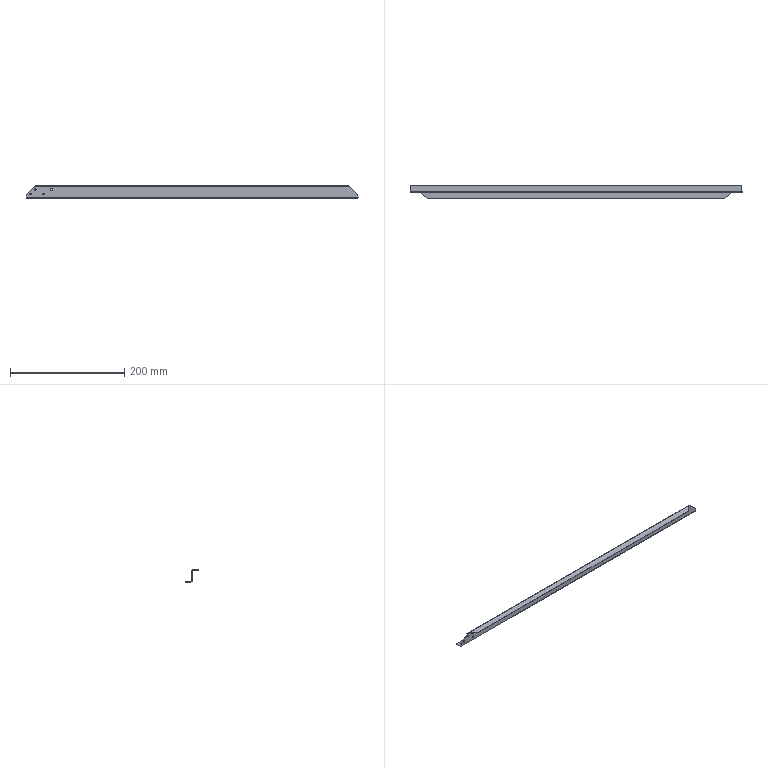Part | SolidWorks | features BaseBody 1 | 1 solid | 28 faces | box 580 x 23.255 x 21.213 mm | volume 12071 mm3 | plane 14 | cylinder 12 | spline 2 | commonest cylinder face diameters 3.2 x8 2 x2 3 x2
STEP:
#1=CARTESIAN_POINT('',(-245.299,-9.6,-7.68));
#2=VERTEX_POINT('',#1);
#3=CARTESIAN_POINT('',(-245.299,-9.556,-4.48));
#4=VERTEX_POINT('',#3);
#5=CARTESIAN_POINT('',(-245.299,-9.578,-6.08));
#6=DIRECTION('',(0.,0.9999,-0.01396));
#7=DIRECTION('',(0.,-0.01396,-0.9999));
#8=AXIS2_PLACEMENT_3D('',#5,#6,#7);
#9=CIRCLE('',#8,1.6);
#10=EDGE_CURVE('',#2,#4,#9,.T.);
#11=ORIENTED_EDGE('',*,*,#10,.T.);
#12=CARTESIAN_POINT('',(-245.299,-10.055,-4.473));
#13=VERTEX_POINT('',#12);
#14=CARTESIAN_POINT('',(-245.299,-9.556,-4.48));
#15=DIRECTION('',(0.,-0.9999,0.01396));
#16=VECTOR('',#15,1000.);
#17=LINE('',#14,#16);
#18=EDGE_CURVE('',#4,#13,#17,.T.);
#19=ORIENTED_EDGE('',*,*,#18,.T.);
#20=CARTESIAN_POINT('',(-245.299,-10.1,-7.673));
#21=VERTEX_POINT('',#20);
#22=CARTESIAN_POINT('',(-245.299,-10.078,-6.073));
#23=DIRECTION('',(0.,-0.9999,0.01396));
#24=DIRECTION('',(0.,-0.01396,-0.9999));
#25=AXIS2_PLACEMENT_3D('',#22,#23,#24);
#26=CIRCLE('',#25,1.6);
#27=EDGE_CURVE('',#13,#21,#26,.T.);
#28=ORIENTED_EDGE('',*,*,#27,.T.);
#29=CARTESIAN_POINT('',(-245.299,-9.6,-7.68));
#30=DIRECTION('',(0.,-0.9999,0.01396));
#31=VECTOR('',#30,1000.);
#32=LINE('',#29,#31);
#33=EDGE_CURVE('',#2,#21,#32,.T.);
#34=ORIENTED_EDGE('',*,*,#33,.F.);
#35=EDGE_LOOP('',(#11,#19,#28,#34));
#36=FACE_OUTER_BOUND('',#35,.T.);
#37=CARTESIAN_POINT('',(-245.299,-9.578,-6.08));
#38=DIRECTION('',(0.,-0.9999,0.01396));
#39=DIRECTION('',(0.,-0.01396,-0.9999));
#40=AXIS2_PLACEMENT_3D('',#37,#38,#39);
#41=CYLINDRICAL_SURFACE('',#40,1.6);
#42=ADVANCED_FACE('',(#36),#41,.F.);
#43=CARTESIAN_POINT('',(-281.91,-9.712,-15.679));
#44=VERTEX_POINT('',#43);
#45=CARTESIAN_POINT('',(-281.91,-9.667,-12.479));
#46=VERTEX_POINT('',#45);
#47=CARTESIAN_POINT('',(-281.91,-9.69,-14.079));
#48=DIRECTION('',(0.,0.9999,-0.01396));
#49=DIRECTION('',(0.,-0.01396,-0.9999));
#50=AXIS2_PLACEMENT_3D('',#47,#48,#49);
#51=CIRCLE('',#50,1.6);
#52=EDGE_CURVE('',#44,#46,#51,.T.);
#53=ORIENTED_EDGE('',*,*,#52,.T.);
#54=CARTESIAN_POINT('',(-281.91,-10.167,-12.472));
#55=VERTEX_POINT('',#54);
#56=CARTESIAN_POINT('',(-281.91,-9.667,-12.479));
#57=DIRECTION('',(0.,-0.9999,0.01396));
#58=VECTOR('',#57,1000.);
#59=LINE('',#56,#58);
#60=EDGE_CURVE('',#46,#55,#59,.T.);
#61=ORIENTED_EDGE('',*,*,#60,.T.);
#62=CARTESIAN_POINT('',(-281.91,-10.212,-15.672));
#63=VERTEX_POINT('',#62);
#64=CARTESIAN_POINT('',(-281.91,-10.19,-14.072));
#65=DIRECTION('',(0.,0.9999,-0.01396));
#66=DIRECTION('',(0.,-0.01396,-0.9999));
#67=AXIS2_PLACEMENT_3D('',#64,#65,#66);
#68=CIRCLE('',#67,1.6);
#69=EDGE_CURVE('',#63,#55,#68,.T.);
#70=ORIENTED_EDGE('',*,*,#69,.F.);
#71=CARTESIAN_POINT('',(-281.91,-9.712,-15.679));
#72=DIRECTION('',(0.,-0.9999,0.01396));
#73=VECTOR('',#72,1000.);
#74=LINE('',#71,#73);
#75=EDGE_CURVE('',#44,#63,#74,.T.);
#76=ORIENTED_EDGE('',*,*,#75,.F.);
#77=EDGE_LOOP('',(#53,#61,#70,#76));
#78=FACE_OUTER_BOUND('',#77,.T.);
#79=CARTESIAN_POINT('',(-281.91,-9.69,-14.079));
#80=DIRECTION('',(0.,-0.9999,0.01396));
#81=DIRECTION('',(0.,-0.01396,-0.9999));
#82=AXIS2_PLACEMENT_3D('',#79,#80,#81);
#83=CYLINDRICAL_SURFACE('',#82,1.6);
#84=ADVANCED_FACE('',(#78),#83,.F.);
#85=CARTESIAN_POINT('',(-273.91,-9.6,-7.68));
#86=VERTEX_POINT('',#85);
#87=CARTESIAN_POINT('',(-273.91,-9.556,-4.48));
#88=VERTEX_POINT('',#87);
#89=CARTESIAN_POINT('',(-273.91,-9.578,-6.08));
#90=DIRECTION('',(0.,0.9999,-0.01396));
#91=DIRECTION('',(0.,-0.01396,-0.9999));
#92=AXIS2_PLACEMENT_3D('',#89,#90,#91);
#93=CIRCLE('',#92,1.6);
#94=EDGE_CURVE('',#86,#88,#93,.T.);
#95=ORIENTED_EDGE('',*,*,#94,.T.);
#96=CARTESIAN_POINT('',(-273.91,-10.055,-4.473));
#97=VERTEX_POINT('',#96);
#98=CARTESIAN_POINT('',(-273.91,-9.556,-4.48));
#99=DIRECTION('',(0.,-0.9999,0.01396));
#100=VECTOR('',#99,1000.);
#101=LINE('',#98,#100);
#102=EDGE_CURVE('',#88,#97,#101,.T.);
#103=ORIENTED_EDGE('',*,*,#102,.T.);
#104=CARTESIAN_POINT('',(-273.91,-10.1,-7.673));
#105=VERTEX_POINT('',#104);
#106=CARTESIAN_POINT('',(-273.91,-10.078,-6.073));
#107=DIRECTION('',(0.,0.9999,-0.01396));
#108=DIRECTION('',(0.,-0.01396,-0.9999));
#109=AXIS2_PLACEMENT_3D('',#106,#107,#108);
#110=CIRCLE('',#109,1.6);
#111=EDGE_CURVE('',#105,#97,#110,.T.);
#112=ORIENTED_EDGE('',*,*,#111,.F.);
#113=CARTESIAN_POINT('',(-273.91,-9.6,-7.68));
#114=DIRECTION('',(0.,-0.9999,0.01396));
#115=VECTOR('',#114,1000.);
#116=LINE('',#113,#115);
#117=EDGE_CURVE('',#86,#105,#116,.T.);
#118=ORIENTED_EDGE('',*,*,#117,.F.);
#119=EDGE_LOOP('',(#95,#103,#112,#118));
#120=FACE_OUTER_BOUND('',#119,.T.);
#121=CARTESIAN_POINT('',(-273.91,-9.578,-6.08));
#122=DIRECTION('',(0.,-0.9999,0.01396));
#123=DIRECTION('',(0.,-0.01396,-0.9999));
#124=AXIS2_PLACEMENT_3D('',#121,#122,#123);
#125=CYLINDRICAL_SURFACE('',#124,1.6);
#126=ADVANCED_FACE('',(#120),#125,.F.);
#127=CARTESIAN_POINT('',(-259.91,-9.712,-15.679));
#128=VERTEX_POINT('',#127);
#129=CARTESIAN_POINT('',(-259.91,-9.667,-12.479));
#130=VERTEX_POINT('',#129);
#131=CARTESIAN_POINT('',(-259.91,-9.69,-14.079));
#132=DIRECTION('',(0.,0.9999,-0.01396));
#133=DIRECTION('',(0.,-0.01396,-0.9999));
#134=AXIS2_PLACEMENT_3D('',#131,#132,#133);
#135=CIRCLE('',#134,1.6);
#136=EDGE_CURVE('',#128,#130,#135,.T.);
#137=ORIENTED_EDGE('',*,*,#136,.T.);
#138=CARTESIAN_POINT('',(-259.91,-10.167,-12.472));
#139=VERTEX_POINT('',#138);
#140=CARTESIAN_POINT('',(-259.91,-9.667,-12.479));
#141=DIRECTION('',(0.,-0.9999,0.01396));
#142=VECTOR('',#141,1000.);
#143=LINE('',#140,#142);
#144=EDGE_CURVE('',#130,#139,#143,.T.);
#145=ORIENTED_EDGE('',*,*,#144,.T.);
#146=CARTESIAN_POINT('',(-259.91,-10.212,-15.672));
#147=VERTEX_POINT('',#146);
#148=CARTESIAN_POINT('',(-259.91,-10.19,-14.072));
#149=DIRECTION('',(0.,0.9999,-0.01396));
#150=DIRECTION('',(0.,-0.01396,-0.9999));
#151=AXIS2_PLACEMENT_3D('',#148,#149,#150);
#152=CIRCLE('',#151,1.6);
#153=EDGE_CURVE('',#147,#139,#152,.T.);
#154=ORIENTED_EDGE('',*,*,#153,.F.);
#155=CARTESIAN_POINT('',(-259.91,-9.712,-15.679));
#156=DIRECTION('',(0.,-0.9999,0.01396));
#157=VECTOR('',#156,1000.);
#158=LINE('',#155,#157);
#159=EDGE_CURVE('',#128,#147,#158,.T.);
#160=ORIENTED_EDGE('',*,*,#159,.F.);
#161=EDGE_LOOP('',(#137,#145,#154,#160));
#162=FACE_OUTER_BOUND('',#161,.T.);
#163=CARTESIAN_POINT('',(-259.91,-9.69,-14.079));
#164=DIRECTION('',(0.,-0.9999,0.01396));
#165=DIRECTION('',(0.,-0.01396,-0.9999));
#166=AXIS2_PLACEMENT_3D('',#163,#164,#165);
#167=CYLINDRICAL_SURFACE('',#166,1.6);
#168=ADVANCED_FACE('',(#162),#167,.F.);
#169=ORIENTED_EDGE('',*,*,#18,.F.);
#170=CARTESIAN_POINT('',(-245.299,-9.578,-6.08));
#171=DIRECTION('',(0.,0.9999,-0.01396));
#172=DIRECTION('',(0.,-0.01396,-0.9999));
#173=AXIS2_PLACEMENT_3D('',#170,#171,#172);
#174=CIRCLE('',#173,1.6);
#175=EDGE_CURVE('',#4,#2,#174,.T.);
#176=ORIENTED_EDGE('',*,*,#175,.T.);
#177=ORIENTED_EDGE('',*,*,#33,.T.);
#178=CARTESIAN_POINT('',(-245.299,-10.078,-6.073));
#179=DIRECTION('',(0.,-0.9999,0.01396));
#180=DIRECTION('',(0.,-0.01396,-0.9999));
#181=AXIS2_PLACEMENT_3D('',#178,#179,#180);
#182=CIRCLE('',#181,1.6);
#183=EDGE_CURVE('',#21,#13,#182,.T.);
#184=ORIENTED_EDGE('',*,*,#183,.T.);
#185=EDGE_LOOP('',(#169,#176,#177,#184));
#186=FACE_OUTER_BOUND('',#185,.T.);
#187=CARTESIAN_POINT('',(-245.299,-9.578,-6.08));
#188=DIRECTION('',(0.,-0.9999,0.01396));
#189=DIRECTION('',(0.,-0.01396,-0.9999));
#190=AXIS2_PLACEMENT_3D('',#187,#188,#189);
#191=CYLINDRICAL_SURFACE('',#190,1.6);
#192=ADVANCED_FACE('',(#186),#191,.F.);
#193=ORIENTED_EDGE('',*,*,#69,.T.);
#194=CARTESIAN_POINT('',(-281.91,-10.19,-14.072));
#195=DIRECTION('',(0.,0.9999,-0.01396));
#196=DIRECTION('',(0.,-0.01396,-0.9999));
#197=AXIS2_PLACEMENT_3D('',#194,#195,#196);
#198=CIRCLE('',#197,1.6);
#199=EDGE_CURVE('',#55,#63,#198,.T.);
#200=ORIENTED_EDGE('',*,*,#199,.T.);
#201=EDGE_LOOP('',(#193,#200));
#202=FACE_BOUND('',#201,.T.);
#203=ORIENTED_EDGE('',*,*,#111,.T.);
#204=CARTESIAN_POINT('',(-273.91,-10.078,-6.073));
#205=DIRECTION('',(0.,0.9999,-0.01396));
#206=DIRECTION('',(0.,-0.01396,-0.9999));
#207=AXIS2_PLACEMENT_3D('',#204,#205,#206);
#208=CIRCLE('',#207,1.6);
#209=EDGE_CURVE('',#97,#105,#208,.T.);
#210=ORIENTED_EDGE('',*,*,#209,.T.);
#211=EDGE_LOOP('',(#203,#210));
#212=FACE_BOUND('',#211,.T.);
#213=ORIENTED_EDGE('',*,*,#153,.T.);
#214=CARTESIAN_POINT('',(-259.91,-10.19,-14.072));
#215=DIRECTION('',(0.,0.9999,-0.01396));
#216=DIRECTION('',(0.,-0.01396,-0.9999));
#217=AXIS2_PLACEMENT_3D('',#214,#215,#216);
#218=CIRCLE('',#217,1.6);
#219=EDGE_CURVE('',#139,#147,#218,.T.);
#220=ORIENTED_EDGE('',*,*,#219,.T.);
#221=EDGE_LOOP('',(#213,#220));
#222=FACE_BOUND('',#221,.T.);
#223=ORIENTED_EDGE('',*,*,#183,.F.);
#224=ORIENTED_EDGE('',*,*,#27,.F.);
#225=EDGE_LOOP('',(#223,#224));
#226=FACE_BOUND('',#225,.T.);
#227=CARTESIAN_POINT('',(290.,-10.266,-19.545));
#228=VERTEX_POINT('',#227);
#229=CARTESIAN_POINT('',(290.,-10.196,-14.546));
#230=VERTEX_POINT('',#229);
#231=CARTESIAN_POINT('',(290.,-10.14,-10.53));
#232=DIRECTION('',(0.,0.01396,0.9999));
#233=VECTOR('',#232,1000.);
#234=LINE('',#231,#233);
#235=EDGE_CURVE('',#228,#230,#234,.T.);
#236=ORIENTED_EDGE('',*,*,#235,.T.);
#237=CARTESIAN_POINT('',(274.653,-10.014,-1.514));
#238=VERTEX_POINT('',#237);
#239=CARTESIAN_POINT('',(290.,-10.196,-14.546));
#240=DIRECTION('',(-0.7622,0.009038,0.6472));
#241=VECTOR('',#240,1000.);
#242=LINE('',#239,#241);
#243=EDGE_CURVE('',#230,#238,#242,.T.);
#244=ORIENTED_EDGE('',*,*,#243,.T.);
#245=CARTESIAN_POINT('',(-274.653,-10.014,-1.514));
#246=VERTEX_POINT('',#245);
#247=CARTESIAN_POINT('',(0.,-10.014,-1.514));
#248=DIRECTION('',(-1.,0.,0.));
#249=VECTOR('',#248,1000.);
#250=LINE('',#247,#249);
#251=EDGE_CURVE('',#238,#246,#250,.T.);
#252=ORIENTED_EDGE('',*,*,#251,.T.);
#253=CARTESIAN_POINT('',(-290.,-10.196,-14.546));
#254=VERTEX_POINT('',#253);
#255=CARTESIAN_POINT('',(-274.653,-10.014,-1.514));
#256=DIRECTION('',(-0.7622,-0.009038,-0.6472));
#257=VECTOR('',#256,1000.);
#258=LINE('',#255,#257);
#259=EDGE_CURVE('',#246,#254,#258,.T.);
#260=ORIENTED_EDGE('',*,*,#259,.T.);
#261=CARTESIAN_POINT('',(-290.,-10.266,-19.545));
#262=VERTEX_POINT('',#261);
#263=CARTESIAN_POINT('',(-290.,-10.14,-10.53));
#264=DIRECTION('',(0.,-0.01396,-0.9999));
#265=VECTOR('',#264,1000.);
#266=LINE('',#263,#265);
#267=EDGE_CURVE('',#254,#262,#266,.T.);
#268=ORIENTED_EDGE('',*,*,#267,.T.);
#269=CARTESIAN_POINT('',(0.,-10.266,-19.545));
#270=DIRECTION('',(1.,0.,0.));
#271=VECTOR('',#270,1000.);
#272=LINE('',#269,#271);
#273=EDGE_CURVE('',#262,#228,#272,.T.);
#274=ORIENTED_EDGE('',*,*,#273,.T.);
#275=EDGE_LOOP('',(#236,#244,#252,#260,#268,#274));
#276=FACE_OUTER_BOUND('',#275,.T.);
#277=CARTESIAN_POINT('',(290.,-10.014,-1.514));
#278=DIRECTION('',(0.,-0.9999,0.01396));
#279=DIRECTION('',(-1.,0.,0.));
#280=AXIS2_PLACEMENT_3D('',#277,#278,#279);
#281=PLANE('',#280);
#282=ADVANCED_FACE('',(#202,#212,#222,#226,#276),#281,.T.);
#283=ORIENTED_EDGE('',*,*,#52,.F.);
#284=CARTESIAN_POINT('',(-281.91,-9.69,-14.079));
#285=DIRECTION('',(0.,0.9999,-0.01396));
#286=DIRECTION('',(0.,-0.01396,-0.9999));
#287=AXIS2_PLACEMENT_3D('',#284,#285,#286);
#288=CIRCLE('',#287,1.6);
#289=EDGE_CURVE('',#46,#44,#288,.T.);
#290=ORIENTED_EDGE('',*,*,#289,.F.);
#291=EDGE_LOOP('',(#283,#290));
#292=FACE_BOUND('',#291,.T.);
#293=ORIENTED_EDGE('',*,*,#94,.F.);
#294=CARTESIAN_POINT('',(-273.91,-9.578,-6.08));
#295=DIRECTION('',(0.,0.9999,-0.01396));
#296=DIRECTION('',(0.,-0.01396,-0.9999));
#297=AXIS2_PLACEMENT_3D('',#294,#295,#296);
#298=CIRCLE('',#297,1.6);
#299=EDGE_CURVE('',#88,#86,#298,.T.);
#300=ORIENTED_EDGE('',*,*,#299,.F.);
#301=EDGE_LOOP('',(#293,#300));
#302=FACE_BOUND('',#301,.T.);
#303=ORIENTED_EDGE('',*,*,#136,.F.);
#304=CARTESIAN_POINT('',(-259.91,-9.69,-14.079));
#305=DIRECTION('',(0.,0.9999,-0.01396));
#306=DIRECTION('',(0.,-0.01396,-0.9999));
#307=AXIS2_PLACEMENT_3D('',#304,#305,#306);
#308=CIRCLE('',#307,1.6);
#309=EDGE_CURVE('',#130,#128,#308,.T.);
#310=ORIENTED_EDGE('',*,*,#309,.F.);
#311=EDGE_LOOP('',(#303,#310));
#312=FACE_BOUND('',#311,.T.);
#313=ORIENTED_EDGE('',*,*,#10,.F.);
#314=ORIENTED_EDGE('',*,*,#175,.F.);
#315=EDGE_LOOP('',(#313,#314));
#316=FACE_BOUND('',#315,.T.);
#317=CARTESIAN_POINT('',(274.653,-9.514,-1.521));
#318=VERTEX_POINT('',#317);
#319=CARTESIAN_POINT('',(-274.653,-9.514,-1.521));
#320=VERTEX_POINT('',#319);
#321=CARTESIAN_POINT('',(0.,-9.514,-1.521));
#322=DIRECTION('',(-1.,0.,0.));
#323=VECTOR('',#322,1000.);
#324=LINE('',#321,#323);
#325=EDGE_CURVE('',#318,#320,#324,.T.);
#326=ORIENTED_EDGE('',*,*,#325,.F.);
#327=CARTESIAN_POINT('',(290.,-9.696,-14.553));
#328=VERTEX_POINT('',#327);
#329=CARTESIAN_POINT('',(274.653,-9.514,-1.521));
#330=DIRECTION('',(-0.7622,0.009038,0.6472));
#331=VECTOR('',#330,1000.);
#332=LINE('',#329,#331);
#333=EDGE_CURVE('',#328,#318,#332,.T.);
#334=ORIENTED_EDGE('',*,*,#333,.F.);
#335=CARTESIAN_POINT('',(290.,-9.766,-19.552));
#336=VERTEX_POINT('',#335);
#337=CARTESIAN_POINT('',(290.,-9.64,-10.537));
#338=DIRECTION('',(0.,0.01396,0.9999));
#339=VECTOR('',#338,1000.);
#340=LINE('',#337,#339);
#341=EDGE_CURVE('',#336,#328,#340,.T.);
#342=ORIENTED_EDGE('',*,*,#341,.F.);
#343=CARTESIAN_POINT('',(-290.,-9.766,-19.552));
#344=VERTEX_POINT('',#343);
#345=CARTESIAN_POINT('',(0.,-9.766,-19.552));
#346=DIRECTION('',(1.,0.,0.));
#347=VECTOR('',#346,1000.);
#348=LINE('',#345,#347);
#349=EDGE_CURVE('',#344,#336,#348,.T.);
#350=ORIENTED_EDGE('',*,*,#349,.F.);
#351=CARTESIAN_POINT('',(-290.,-9.696,-14.553));
#352=VERTEX_POINT('',#351);
#353=CARTESIAN_POINT('',(-290.,-9.64,-10.537));
#354=DIRECTION('',(0.,-0.01396,-0.9999));
#355=VECTOR('',#354,1000.);
#356=LINE('',#353,#355);
#357=EDGE_CURVE('',#352,#344,#356,.T.);
#358=ORIENTED_EDGE('',*,*,#357,.F.);
#359=CARTESIAN_POINT('',(-290.,-9.696,-14.553));
#360=DIRECTION('',(-0.7622,-0.009038,-0.6472));
#361=VECTOR('',#360,1000.);
#362=LINE('',#359,#361);
#363=EDGE_CURVE('',#320,#352,#362,.T.);
#364=ORIENTED_EDGE('',*,*,#363,.F.);
#365=EDGE_LOOP('',(#326,#334,#342,#350,#358,#364));
#366=FACE_OUTER_BOUND('',#365,.T.);
#367=CARTESIAN_POINT('',(290.,-9.514,-1.521));
#368=DIRECTION('',(0.,-0.9999,0.01396));
#369=DIRECTION('',(-1.,0.,0.));
#370=AXIS2_PLACEMENT_3D('',#367,#368,#369);
#371=PLANE('',#370);
#372=ADVANCED_FACE('',(#292,#302,#312,#316,#366),#371,.F.);
#373=ORIENTED_EDGE('',*,*,#60,.F.);
#374=ORIENTED_EDGE('',*,*,#289,.T.);
#375=ORIENTED_EDGE('',*,*,#75,.T.);
#376=ORIENTED_EDGE('',*,*,#199,.F.);
#377=EDGE_LOOP('',(#373,#374,#375,#376));
#378=FACE_OUTER_BOUND('',#377,.T.);
#379=CARTESIAN_POINT('',(-281.91,-9.69,-14.079));
#380=DIRECTION('',(0.,-0.9999,0.01396));
#381=DIRECTION('',(0.,-0.01396,-0.9999));
#382=AXIS2_PLACEMENT_3D('',#379,#380,#381);
#383=CYLINDRICAL_SURFACE('',#382,1.6);
#384=ADVANCED_FACE('',(#378),#383,.F.);
#385=ORIENTED_EDGE('',*,*,#102,.F.);
#386=ORIENTED_EDGE('',*,*,#299,.T.);
#387=ORIENTED_EDGE('',*,*,#117,.T.);
#388=ORIENTED_EDGE('',*,*,#209,.F.);
#389=EDGE_LOOP('',(#385,#386,#387,#388));
#390=FACE_OUTER_BOUND('',#389,.T.);
#391=CARTESIAN_POINT('',(-273.91,-9.578,-6.08));
#392=DIRECTION('',(0.,-0.9999,0.01396));
#393=DIRECTION('',(0.,-0.01396,-0.9999));
#394=AXIS2_PLACEMENT_3D('',#391,#392,#393);
#395=CYLINDRICAL_SURFACE('',#394,1.6);
#396=ADVANCED_FACE('',(#390),#395,.F.);
#397=ORIENTED_EDGE('',*,*,#144,.F.);
#398=ORIENTED_EDGE('',*,*,#309,.T.);
#399=ORIENTED_EDGE('',*,*,#159,.T.);
#400=ORIENTED_EDGE('',*,*,#219,.F.);
#401=EDGE_LOOP('',(#397,#398,#399,#400));
#402=FACE_OUTER_BOUND('',#401,.T.);
#403=CARTESIAN_POINT('',(-259.91,-9.69,-14.079));
#404=DIRECTION('',(0.,-0.9999,0.01396));
#405=DIRECTION('',(0.,-0.01396,-0.9999));
#406=AXIS2_PLACEMENT_3D('',#403,#404,#405);
#407=CYLINDRICAL_SURFACE('',#406,1.6);
#408=ADVANCED_FACE('',(#402),#407,.F.);
#409=CARTESIAN_POINT('',(290.,-9.946,-14.549));
#410=DIRECTION('',(0.,0.9999,-0.01396));
#411=VECTOR('',#410,1000.);
#412=LINE('',#409,#411);
#413=EDGE_CURVE('',#230,#328,#412,.T.);
#414=ORIENTED_EDGE('',*,*,#413,.T.);
#415=ORIENTED_EDGE('',*,*,#333,.T.);
#416=CARTESIAN_POINT('',(274.653,-9.764,-1.517));
#417=DIRECTION('',(0.,-0.9999,0.01396));
#418=VECTOR('',#417,1000.);
#419=LINE('',#416,#418);
#420=EDGE_CURVE('',#318,#238,#419,.T.);
#421=ORIENTED_EDGE('',*,*,#420,.T.);
#422=ORIENTED_EDGE('',*,*,#243,.F.);
#423=EDGE_LOOP('',(#414,#415,#421,#422));
#424=FACE_OUTER_BOUND('',#423,.T.);
#425=CARTESIAN_POINT('',(274.653,-10.014,-1.514));
#426=DIRECTION('',(0.6473,0.01064,0.7622));
#427=DIRECTION('',(0.7622,-0.009038,-0.6472));
#428=AXIS2_PLACEMENT_3D('',#425,#426,#427);
#429=PLANE('',#428);
#430=ADVANCED_FACE('',(#424),#429,.T.);
#431=ORIENTED_EDGE('',*,*,#341,.T.);
#432=ORIENTED_EDGE('',*,*,#413,.F.);
#433=ORIENTED_EDGE('',*,*,#235,.F.);
#434=CARTESIAN_POINT('',(290.,-8.787,-21.066));
#435=VERTEX_POINT('',#434);
#436=CARTESIAN_POINT('',(290.,-8.766,-19.566));
#437=DIRECTION('',(1.,0.,0.));
#438=DIRECTION('',(0.,0.,-1.));
#439=AXIS2_PLACEMENT_3D('',#436,#437,#438);
#440=CIRCLE('',#439,1.5);
#441=EDGE_CURVE('',#228,#435,#440,.T.);
#442=ORIENTED_EDGE('',*,*,#441,.T.);
#443=CARTESIAN_POINT('',(290.,1.748,-21.213));
#444=VERTEX_POINT('',#443);
#445=CARTESIAN_POINT('',(290.,-3.519,-21.14));
#446=DIRECTION('',(0.,-0.9999,0.01396));
#447=VECTOR('',#446,1000.);
#448=LINE('',#445,#447);
#449=EDGE_CURVE('',#444,#435,#448,.T.);
#450=ORIENTED_EDGE('',*,*,#449,.F.);
#451=CARTESIAN_POINT('',(290.,1.755,-20.713));
#452=VERTEX_POINT('',#451);
#453=CARTESIAN_POINT('',(290.,1.752,-20.963));
#454=DIRECTION('',(0.,0.01396,0.9999));
#455=VECTOR('',#454,1000.);
#456=LINE('',#453,#455);
#457=EDGE_CURVE('',#444,#452,#456,.T.);
#458=ORIENTED_EDGE('',*,*,#457,.T.);
#459=CARTESIAN_POINT('',(290.,-8.78,-20.566));
#460=VERTEX_POINT('',#459);
#461=CARTESIAN_POINT('',(290.,-3.512,-20.64));
#462=DIRECTION('',(0.,-0.9999,0.01396));
#463=VECTOR('',#462,1000.);
#464=LINE('',#461,#463);
#465=EDGE_CURVE('',#452,#460,#464,.T.);
#466=ORIENTED_EDGE('',*,*,#465,.T.);
#467=CARTESIAN_POINT('',(290.,-8.766,-19.566));
#468=DIRECTION('',(1.,0.,0.));
#469=DIRECTION('',(0.,0.,-1.));
#470=AXIS2_PLACEMENT_3D('',#467,#468,#469);
#471=CIRCLE('',#470,1.);
#472=EDGE_CURVE('',#336,#460,#471,.T.);
#473=ORIENTED_EDGE('',*,*,#472,.F.);
#474=EDGE_LOOP('',(#431,#432,#433,#442,#450,#458,#466,#473));
#475=FACE_OUTER_BOUND('',#474,.T.);
#476=CARTESIAN_POINT('',(290.,-9.696,-14.553));
#477=DIRECTION('',(1.,0.,0.));
#478=DIRECTION('',(0.,-0.9999,0.01396));
#479=AXIS2_PLACEMENT_3D('',#476,#477,#478);
#480=PLANE('',#479);
#481=ADVANCED_FACE('',(#475),#480,.T.);
#482=ORIENTED_EDGE('',*,*,#273,.F.);
#483=CARTESIAN_POINT('',(-290.,-8.787,-21.066));
#484=VERTEX_POINT('',#483);
#485=CARTESIAN_POINT('',(-290.,-8.766,-19.566));
#486=DIRECTION('',(-1.,0.,0.));
#487=DIRECTION('',(0.,0.,-1.));
#488=AXIS2_PLACEMENT_3D('',#485,#486,#487);
#489=CIRCLE('',#488,1.5);
#490=EDGE_CURVE('',#484,#262,#489,.T.);
#491=ORIENTED_EDGE('',*,*,#490,.F.);
#492=CARTESIAN_POINT('',(0.,-8.787,-21.066));
#493=DIRECTION('',(-1.,0.,0.));
#494=VECTOR('',#493,1000.);
#495=LINE('',#492,#494);
#496=EDGE_CURVE('',#435,#484,#495,.T.);
#497=ORIENTED_EDGE('',*,*,#496,.F.);
#498=ORIENTED_EDGE('',*,*,#441,.F.);
#499=EDGE_LOOP('',(#482,#491,#497,#498));
#500=FACE_OUTER_BOUND('',#499,.T.);
#501=CARTESIAN_POINT('',(-290.,-8.766,-19.566));
#502=DIRECTION('',(1.,0.,0.));
#503=DIRECTION('',(0.,0.,-1.));
#504=AXIS2_PLACEMENT_3D('',#501,#502,#503);
#505=CYLINDRICAL_SURFACE('',#504,1.5);
#506=ADVANCED_FACE('',(#500),#505,.T.);
#507=ORIENTED_EDGE('',*,*,#267,.F.);
#508=CARTESIAN_POINT('',(-290.,-9.946,-14.549));
#509=DIRECTION('',(0.,0.9999,-0.01396));
#510=VECTOR('',#509,1000.);
#511=LINE('',#508,#510);
#512=EDGE_CURVE('',#254,#352,#511,.T.);
#513=ORIENTED_EDGE('',*,*,#512,.T.);
#514=ORIENTED_EDGE('',*,*,#357,.T.);
#515=CARTESIAN_POINT('',(-290.,-8.78,-20.566));
#516=VERTEX_POINT('',#515);
#517=CARTESIAN_POINT('',(-290.,-8.766,-19.566));
#518=DIRECTION('',(-1.,0.,0.));
#519=DIRECTION('',(0.,0.,-1.));
#520=AXIS2_PLACEMENT_3D('',#517,#518,#519);
#521=CIRCLE('',#520,1.);
#522=EDGE_CURVE('',#516,#344,#521,.T.);
#523=ORIENTED_EDGE('',*,*,#522,.F.);
#524=CARTESIAN_POINT('',(-290.,1.755,-20.713));
#525=VERTEX_POINT('',#524);
#526=CARTESIAN_POINT('',(-290.,-3.512,-20.64));
#527=DIRECTION('',(0.,0.9999,-0.01396));
#528=VECTOR('',#527,1000.);
#529=LINE('',#526,#528);
#530=EDGE_CURVE('',#516,#525,#529,.T.);
#531=ORIENTED_EDGE('',*,*,#530,.T.);
#532=CARTESIAN_POINT('',(-290.,1.748,-21.213));
#533=VERTEX_POINT('',#532);
#534=CARTESIAN_POINT('',(-290.,1.752,-20.963));
#535=DIRECTION('',(0.,0.01396,0.9999));
#536=VECTOR('',#535,1000.);
#537=LINE('',#534,#536);
#538=EDGE_CURVE('',#533,#525,#537,.T.);
#539=ORIENTED_EDGE('',*,*,#538,.F.);
#540=CARTESIAN_POINT('',(-290.,-3.519,-21.14));
#541=DIRECTION('',(0.,0.9999,-0.01396));
#542=VECTOR('',#541,1000.);
#543=LINE('',#540,#542);
#544=EDGE_CURVE('',#484,#533,#543,.T.);
#545=ORIENTED_EDGE('',*,*,#544,.F.);
#546=ORIENTED_EDGE('',*,*,#490,.T.);
#547=EDGE_LOOP('',(#507,#513,#514,#523,#531,#539,#545,#546));
#548=FACE_OUTER_BOUND('',#547,.T.);
#549=CARTESIAN_POINT('',(-290.,-10.196,-14.546));
#550=DIRECTION('',(-1.,0.,0.));
#551=DIRECTION('',(0.,0.9999,-0.01396));
#552=AXIS2_PLACEMENT_3D('',#549,#550,#551);
#553=PLANE('',#552);
#554=ADVANCED_FACE('',(#548),#553,.T.);
#555=ORIENTED_EDGE('',*,*,#512,.F.);
#556=ORIENTED_EDGE('',*,*,#259,.F.);
#557=CARTESIAN_POINT('',(-274.653,-9.764,-1.517));
#558=DIRECTION('',(0.,0.9999,-0.01396));
#559=VECTOR('',#558,1000.);
#560=LINE('',#557,#559);
#561=EDGE_CURVE('',#246,#320,#560,.T.);
#562=ORIENTED_EDGE('',*,*,#561,.T.);
#563=ORIENTED_EDGE('',*,*,#363,.T.);
#564=EDGE_LOOP('',(#555,#556,#562,#563));
#565=FACE_OUTER_BOUND('',#564,.T.);
#566=CARTESIAN_POINT('',(-290.,-10.196,-14.546));
#567=DIRECTION('',(-0.6473,0.01064,0.7622));
#568=DIRECTION('',(0.7622,0.009038,0.6472));
#569=AXIS2_PLACEMENT_3D('',#566,#567,#568);
#570=PLANE('',#569);
#571=ADVANCED_FACE('',(#565),#570,.T.);
#572=ORIENTED_EDGE('',*,*,#251,.F.);
#573=CARTESIAN_POINT('',(274.632,-10.014,-1.5));
#574=VERTEX_POINT('',#573);
#575=CARTESIAN_POINT('',(274.653,-10.014,-1.514));
#576=CARTESIAN_POINT('',(274.646,-10.014,-1.509));
#577=CARTESIAN_POINT('',(274.639,-10.014,-1.505));
#578=CARTESIAN_POINT('',(274.632,-10.014,-1.5));
#579=B_SPLINE_CURVE_WITH_KNOTS('',3,(#575,#576,#577,#578),.UNSPECIFIED.,.F.,.F.,(4,4),(0.,1.),.UNSPECIFIED.);
#580=EDGE_CURVE('',#238,#574,#579,.T.);
#581=ORIENTED_EDGE('',*,*,#580,.T.);
#582=CARTESIAN_POINT('',(272.32,-11.014,-0.5));
#583=VERTEX_POINT('',#582);
#584=CARTESIAN_POINT('',(274.632,-10.014,-1.5));
#585=CARTESIAN_POINT('',(274.438,-10.014,-1.368));
#586=CARTESIAN_POINT('',(274.247,-10.04,-1.239));
#587=CARTESIAN_POINT('',(273.863,-10.14,-0.9976));
#588=CARTESIAN_POINT('',(273.669,-10.214,-0.8855));
#589=CARTESIAN_POINT('',(273.285,-10.399,-0.7011));
#590=CARTESIAN_POINT('',(273.094,-10.509,-0.6271));
#591=CARTESIAN_POINT('',(272.706,-10.752,-0.526));
#592=CARTESIAN_POINT('',(272.514,-10.882,-0.5));
#593=CARTESIAN_POINT('',(272.32,-11.014,-0.5));
#594=B_SPLINE_CURVE_WITH_KNOTS('',3,(#584,#585,#586,#587,#588,#589,#590,#591,#592,#593),.UNSPECIFIED.,.F.,.F.,(4,2,2,2,4),(0.,0.000695,0.00139,0.002085,0.00278),.UNSPECIFIED.);
#595=EDGE_CURVE('',#574,#583,#594,.T.);
#596=ORIENTED_EDGE('',*,*,#595,.T.);
#597=CARTESIAN_POINT('',(-272.32,-11.014,-0.5));
#598=VERTEX_POINT('',#597);
#599=CARTESIAN_POINT('',(0.,-11.014,-0.5));
#600=DIRECTION('',(-1.,0.,0.));
#601=VECTOR('',#600,1000.);
#602=LINE('',#599,#601);
#603=EDGE_CURVE('',#583,#598,#602,.T.);
#604=ORIENTED_EDGE('',*,*,#603,.T.);
#605=CARTESIAN_POINT('',(-274.632,-10.014,-1.5));
#606=VERTEX_POINT('',#605);
#607=CARTESIAN_POINT('',(-272.32,-11.014,-0.5));
#608=CARTESIAN_POINT('',(-272.514,-10.882,-0.5));
#609=CARTESIAN_POINT('',(-272.705,-10.753,-0.526));
#610=CARTESIAN_POINT('',(-273.089,-10.512,-0.6256));
#611=CARTESIAN_POINT('',(-273.284,-10.4,-0.7004));
#612=CARTESIAN_POINT('',(-273.667,-10.215,-0.8846));
#613=CARTESIAN_POINT('',(-273.859,-10.141,-0.9947));
#614=CARTESIAN_POINT('',(-274.246,-10.04,-1.238));
#615=CARTESIAN_POINT('',(-274.438,-10.014,-1.368));
#616=CARTESIAN_POINT('',(-274.632,-10.014,-1.5));
#617=B_SPLINE_CURVE_WITH_KNOTS('',3,(#607,#608,#609,#610,#611,#612,#613,#614,#615,#616),.UNSPECIFIED.,.F.,.F.,(4,2,2,2,4),(0.,0.000695,0.00139,0.002085,0.00278),.UNSPECIFIED.);
#618=EDGE_CURVE('',#598,#606,#617,.T.);
#619=ORIENTED_EDGE('',*,*,#618,.T.);
#620=CARTESIAN_POINT('',(-274.632,-10.014,-1.5));
#621=CARTESIAN_POINT('',(-274.639,-10.014,-1.505));
#622=CARTESIAN_POINT('',(-274.646,-10.014,-1.509));
#623=CARTESIAN_POINT('',(-274.653,-10.014,-1.514));
#624=B_SPLINE_CURVE_WITH_KNOTS('',3,(#620,#621,#622,#623),.UNSPECIFIED.,.F.,.F.,(4,4),(0.,1.),.UNSPECIFIED.);
#625=EDGE_CURVE('',#606,#246,#624,.T.);
#626=ORIENTED_EDGE('',*,*,#625,.T.);
#627=EDGE_LOOP('',(#572,#581,#596,#604,#619,#626));
#628=FACE_OUTER_BOUND('',#627,.T.);
#629=CARTESIAN_POINT('',(-277.949,-11.014,-1.5));
#630=DIRECTION('',(1.,0.,0.));
#631=DIRECTION('',(0.,0.,-1.));
#632=AXIS2_PLACEMENT_3D('',#629,#630,#631);
#633=CYLINDRICAL_SURFACE('',#632,1.);
#634=ADVANCED_FACE('',(#628),#633,.F.);
#635=CARTESIAN_POINT('',(-274.632,-9.514,-1.5));
#636=VERTEX_POINT('',#635);
#637=CARTESIAN_POINT('',(-274.653,-9.514,-1.521));
#638=CARTESIAN_POINT('',(-274.646,-9.514,-1.514));
#639=CARTESIAN_POINT('',(-274.639,-9.514,-1.507));
#640=CARTESIAN_POINT('',(-274.632,-9.514,-1.5));
#641=B_SPLINE_CURVE_WITH_KNOTS('',3,(#637,#638,#639,#640),.UNSPECIFIED.,.F.,.F.,(4,4),(0.,1.),.UNSPECIFIED.);
#642=EDGE_CURVE('',#320,#636,#641,.T.);
#643=ORIENTED_EDGE('',*,*,#642,.T.);
#644=CARTESIAN_POINT('',(-272.32,-11.014,0.));
#645=VERTEX_POINT('',#644);
#646=CARTESIAN_POINT('',(-272.32,-11.014,0.));
#647=CARTESIAN_POINT('',(-272.514,-10.816,-0.000000003));
#648=CARTESIAN_POINT('',(-272.704,-10.623,-0.03871));
#649=CARTESIAN_POINT('',(-272.993,-10.35,-0.1513));
#650=CARTESIAN_POINT('',(-273.091,-10.262,-0.1983));
#651=CARTESIAN_POINT('',(-273.283,-10.099,-0.3072));
#652=CARTESIAN_POINT('',(-273.379,-10.024,-0.3693));
#653=CARTESIAN_POINT('',(-273.667,-9.816,-0.5765));
#654=CARTESIAN_POINT('',(-273.861,-9.704,-0.7444));
#655=CARTESIAN_POINT('',(-274.244,-9.554,-1.105));
#656=CARTESIAN_POINT('',(-274.438,-9.514,-1.302));
#657=CARTESIAN_POINT('',(-274.632,-9.514,-1.5));
#658=B_SPLINE_CURVE_WITH_KNOTS('',3,(#646,#647,#648,#649,#650,#651,#652,#653,#654,#655,#656,#657),.UNSPECIFIED.,.F.,.F.,(4,2,2,2,2,4),(0.,0.0008207,0.001231,0.001641,0.002462,0.003283),.UNSPECIFIED.);
#659=EDGE_CURVE('',#645,#636,#658,.T.);
#660=ORIENTED_EDGE('',*,*,#659,.F.);
#661=CARTESIAN_POINT('',(272.32,-11.014,0.));
#662=VERTEX_POINT('',#661);
#663=CARTESIAN_POINT('',(0.,-11.014,0.));
#664=DIRECTION('',(-1.,0.,0.));
#665=VECTOR('',#664,1000.);
#666=LINE('',#663,#665);
#667=EDGE_CURVE('',#662,#645,#666,.T.);
#668=ORIENTED_EDGE('',*,*,#667,.F.);
#669=CARTESIAN_POINT('',(274.632,-9.514,-1.5));
#670=VERTEX_POINT('',#669);
#671=CARTESIAN_POINT('',(274.632,-9.514,-1.5));
#672=CARTESIAN_POINT('',(274.438,-9.514,-1.302));
#673=CARTESIAN_POINT('',(274.248,-9.553,-1.109));
#674=CARTESIAN_POINT('',(273.959,-9.665,-0.8362));
#675=CARTESIAN_POINT('',(273.861,-9.712,-0.7482));
#676=CARTESIAN_POINT('',(273.669,-9.821,-0.5852));
#677=CARTESIAN_POINT('',(273.573,-9.883,-0.5095));
#678=CARTESIAN_POINT('',(273.286,-10.091,-0.3019));
#679=CARTESIAN_POINT('',(273.091,-10.258,-0.1896));
#680=CARTESIAN_POINT('',(272.708,-10.619,-0.03982));
#681=CARTESIAN_POINT('',(272.514,-10.816,-0.000000003));
#682=CARTESIAN_POINT('',(272.32,-11.014,0.));
#683=B_SPLINE_CURVE_WITH_KNOTS('',3,(#671,#672,#673,#674,#675,#676,#677,#678,#679,#680,#681,#682),.UNSPECIFIED.,.F.,.F.,(4,2,2,2,2,4),(0.,0.0008207,0.001231,0.001641,0.002462,0.003283),.UNSPECIFIED.);
#684=EDGE_CURVE('',#670,#662,#683,.T.);
#685=ORIENTED_EDGE('',*,*,#684,.F.);
#686=CARTESIAN_POINT('',(274.632,-9.514,-1.5));
#687=CARTESIAN_POINT('',(274.639,-9.514,-1.507));
#688=CARTESIAN_POINT('',(274.646,-9.514,-1.514));
#689=CARTESIAN_POINT('',(274.653,-9.514,-1.521));
#690=B_SPLINE_CURVE_WITH_KNOTS('',3,(#686,#687,#688,#689),.UNSPECIFIED.,.F.,.F.,(4,4),(0.,1.),.UNSPECIFIED.);
#691=EDGE_CURVE('',#670,#318,#690,.T.);
#692=ORIENTED_EDGE('',*,*,#691,.T.);
#693=ORIENTED_EDGE('',*,*,#325,.T.);
#694=EDGE_LOOP('',(#643,#660,#668,#685,#692,#693));
#695=FACE_OUTER_BOUND('',#694,.T.);
#696=CARTESIAN_POINT('',(-277.949,-11.014,-1.5));
#697=DIRECTION('',(1.,0.,0.));
#698=DIRECTION('',(0.,0.,-1.));
#699=AXIS2_PLACEMENT_3D('',#696,#697,#698);
#700=CYLINDRICAL_SURFACE('',#699,1.5);
#701=ADVANCED_FACE('',(#695),#700,.T.);
#702=ORIENTED_EDGE('',*,*,#522,.T.);
#703=ORIENTED_EDGE('',*,*,#349,.T.);
#704=ORIENTED_EDGE('',*,*,#472,.T.);
#705=CARTESIAN_POINT('',(0.,-8.78,-20.566));
#706=DIRECTION('',(-1.,0.,0.));
#707=VECTOR('',#706,1000.);
#708=LINE('',#705,#707);
#709=EDGE_CURVE('',#460,#516,#708,.T.);
#710=ORIENTED_EDGE('',*,*,#709,.T.);
#711=EDGE_LOOP('',(#702,#703,#704,#710));
#712=FACE_OUTER_BOUND('',#711,.T.);
#713=CARTESIAN_POINT('',(-290.,-8.766,-19.566));
#714=DIRECTION('',(1.,0.,0.));
#715=DIRECTION('',(0.,0.,-1.));
#716=AXIS2_PLACEMENT_3D('',#713,#714,#715);
#717=CYLINDRICAL_SURFACE('',#716,1.);
#718=ADVANCED_FACE('',(#712),#717,.F.);
#719=CARTESIAN_POINT('',(0.,1.748,-21.213));
#720=DIRECTION('',(1.,0.,0.));
#721=VECTOR('',#720,1000.);
#722=LINE('',#719,#721);
#723=EDGE_CURVE('',#533,#444,#722,.T.);
#724=ORIENTED_EDGE('',*,*,#723,.T.);
#725=ORIENTED_EDGE('',*,*,#449,.T.);
#726=ORIENTED_EDGE('',*,*,#496,.T.);
#727=ORIENTED_EDGE('',*,*,#544,.T.);
#728=EDGE_LOOP('',(#724,#725,#726,#727));
#729=FACE_OUTER_BOUND('',#728,.T.);
#730=CARTESIAN_POINT('',(290.,-8.787,-21.066));
#731=DIRECTION('',(0.,-0.01396,-0.9999));
#732=DIRECTION('',(-1.,0.,0.));
#733=AXIS2_PLACEMENT_3D('',#730,#731,#732);
#734=PLANE('',#733);
#735=ADVANCED_FACE('',(#729),#734,.T.);
#736=ORIENTED_EDGE('',*,*,#709,.F.);
#737=ORIENTED_EDGE('',*,*,#465,.F.);
#738=CARTESIAN_POINT('',(0.,1.755,-20.713));
#739=DIRECTION('',(1.,0.,0.));
#740=VECTOR('',#739,1000.);
#741=LINE('',#738,#740);
#742=EDGE_CURVE('',#525,#452,#741,.T.);
#743=ORIENTED_EDGE('',*,*,#742,.F.);
#744=ORIENTED_EDGE('',*,*,#530,.F.);
#745=EDGE_LOOP('',(#736,#737,#743,#744));
#746=FACE_OUTER_BOUND('',#745,.T.);
#747=CARTESIAN_POINT('',(290.,-8.78,-20.566));
#748=DIRECTION('',(0.,-0.01396,-0.9999));
#749=DIRECTION('',(-1.,0.,0.));
#750=AXIS2_PLACEMENT_3D('',#747,#748,#749);
#751=PLANE('',#750);
#752=ADVANCED_FACE('',(#746),#751,.F.);
#753=ORIENTED_EDGE('',*,*,#723,.F.);
#754=ORIENTED_EDGE('',*,*,#538,.T.);
#755=ORIENTED_EDGE('',*,*,#742,.T.);
#756=ORIENTED_EDGE('',*,*,#457,.F.);
#757=EDGE_LOOP('',(#753,#754,#755,#756));
#758=FACE_OUTER_BOUND('',#757,.T.);
#759=CARTESIAN_POINT('',(290.,1.748,-21.213));
#760=DIRECTION('',(0.,0.9999,-0.01396));
#761=DIRECTION('',(-1.,0.,0.));
#762=AXIS2_PLACEMENT_3D('',#759,#760,#761);
#763=PLANE('',#762);
#764=ADVANCED_FACE('',(#758),#763,.T.);
#765=CARTESIAN_POINT('',(259.972,-21.5,-0.5));
#766=VERTEX_POINT('',#765);
#767=CARTESIAN_POINT('',(272.32,-11.014,-0.5));
#768=DIRECTION('',(-0.7622,-0.6473,0.));
#769=VECTOR('',#768,1000.);
#770=LINE('',#767,#769);
#771=EDGE_CURVE('',#583,#766,#770,.T.);
#772=ORIENTED_EDGE('',*,*,#771,.T.);
#773=CARTESIAN_POINT('',(-259.972,-21.5,-0.5));
#774=VERTEX_POINT('',#773);
#775=CARTESIAN_POINT('',(0.,-21.5,-0.5));
#776=DIRECTION('',(-1.,0.,0.));
#777=VECTOR('',#776,1000.);
#778=LINE('',#775,#777);
#779=EDGE_CURVE('',#766,#774,#778,.T.);
#780=ORIENTED_EDGE('',*,*,#779,.T.);
#781=CARTESIAN_POINT('',(-259.972,-21.5,-0.5));
#782=DIRECTION('',(-0.7622,0.6473,0.));
#783=VECTOR('',#782,1000.);
#784=LINE('',#781,#783);
#785=EDGE_CURVE('',#774,#598,#784,.T.);
#786=ORIENTED_EDGE('',*,*,#785,.T.);
#787=ORIENTED_EDGE('',*,*,#603,.F.);
#788=EDGE_LOOP('',(#772,#780,#786,#787));
#789=FACE_OUTER_BOUND('',#788,.T.);
#790=CARTESIAN_POINT('',(275.588,-21.5,-0.5));
#791=DIRECTION('',(0.,0.,-1.));
#792=DIRECTION('',(-1.,0.,0.));
#793=AXIS2_PLACEMENT_3D('',#790,#791,#792);
#794=PLANE('',#793);
#795=ADVANCED_FACE('',(#789),#794,.T.);
#796=ORIENTED_EDGE('',*,*,#691,.F.);
#797=ORIENTED_EDGE('',*,*,#684,.T.);
#798=CARTESIAN_POINT('',(272.32,-11.014,-0.25));
#799=DIRECTION('',(0.,0.,1.));
#800=VECTOR('',#799,1000.);
#801=LINE('',#798,#800);
#802=EDGE_CURVE('',#583,#662,#801,.T.);
#803=ORIENTED_EDGE('',*,*,#802,.F.);
#804=ORIENTED_EDGE('',*,*,#595,.F.);
#805=ORIENTED_EDGE('',*,*,#580,.F.);
#806=ORIENTED_EDGE('',*,*,#420,.F.);
#807=EDGE_LOOP('',(#796,#797,#803,#804,#805,#806));
#808=FACE_OUTER_BOUND('',#807,.T.);
#809=CARTESIAN_POINT('',(274.653,-9.509,-1.521));
#810=CARTESIAN_POINT('',(274.458,-9.506,-1.322));
#811=CARTESIAN_POINT('',(274.264,-9.543,-1.123));
#812=CARTESIAN_POINT('',(273.875,-9.692,-0.7542));
#813=CARTESIAN_POINT('',(273.681,-9.803,-0.5847));
#814=CARTESIAN_POINT('',(273.292,-10.082,-0.3017));
#815=CARTESIAN_POINT('',(273.098,-10.25,-0.1882));
#816=CARTESIAN_POINT('',(272.709,-10.617,-0.03483));
#817=CARTESIAN_POINT('',(272.514,-10.815,0.00505));
#818=CARTESIAN_POINT('',(272.32,-11.014,0.00505));
#819=CARTESIAN_POINT('',(274.653,-9.514,-1.521));
#820=CARTESIAN_POINT('',(274.458,-9.511,-1.323));
#821=CARTESIAN_POINT('',(274.264,-9.548,-1.124));
#822=CARTESIAN_POINT('',(273.875,-9.696,-0.7567));
#823=CARTESIAN_POINT('',(273.681,-9.807,-0.5878));
#824=CARTESIAN_POINT('',(273.292,-10.085,-0.3057));
#825=CARTESIAN_POINT('',(273.098,-10.252,-0.1926));
#826=CARTESIAN_POINT('',(272.709,-10.618,-0.03975));
#827=CARTESIAN_POINT('',(272.514,-10.816,0.));
#828=CARTESIAN_POINT('',(272.32,-11.014,0.));
#829=CARTESIAN_POINT('',(274.653,-10.014,-1.514));
#830=CARTESIAN_POINT('',(274.458,-10.012,-1.382));
#831=CARTESIAN_POINT('',(274.264,-10.037,-1.25));
#832=CARTESIAN_POINT('',(273.875,-10.135,-1.004));
#833=CARTESIAN_POINT('',(273.681,-10.209,-0.8919));
#834=CARTESIAN_POINT('',(273.292,-10.395,-0.7038));
#835=CARTESIAN_POINT('',(273.098,-10.506,-0.6284));
#836=CARTESIAN_POINT('',(272.709,-10.75,-0.5265));
#837=CARTESIAN_POINT('',(272.514,-10.882,-0.5));
#838=CARTESIAN_POINT('',(272.32,-11.014,-0.5));
#839=CARTESIAN_POINT('',(274.653,-10.019,-1.514));
#840=CARTESIAN_POINT('',(274.458,-10.017,-1.382));
#841=CARTESIAN_POINT('',(274.264,-10.042,-1.251));
#842=CARTESIAN_POINT('',(273.875,-10.14,-1.007));
#843=CARTESIAN_POINT('',(273.681,-10.213,-0.8949));
#844=CARTESIAN_POINT('',(273.292,-10.398,-0.7078));
#845=CARTESIAN_POINT('',(273.098,-10.509,-0.6328));
#846=CARTESIAN_POINT('',(272.709,-10.751,-0.5314));
#847=CARTESIAN_POINT('',(272.514,-10.883,-0.505));
#848=CARTESIAN_POINT('',(272.32,-11.014,-0.505));
#849=B_SPLINE_SURFACE_WITH_KNOTS('',1,3,((#809,#810,#811,#812,#813,#814,#815,#816,#817,#818),(#819,#820,#821,#822,#823,#824,#825,#826,#827,#828),(#829,#830,#831,#832,#833,#834,#835,#836,#837,#838),(#839,#840,#841,#842,#843,#844,#845,#846,#847,#848)),.UNSPECIFIED.,.F.,.F.,.F.,(2,1,1,2),(4,2,2,2,4),(-0.0101,0.,1.,1.01),(0.,0.25,0.5,0.75,1.),.UNSPECIFIED.);
#850=ADVANCED_FACE('',(#808),#849,.F.);
#851=ORIENTED_EDGE('',*,*,#659,.T.);
#852=ORIENTED_EDGE('',*,*,#642,.F.);
#853=ORIENTED_EDGE('',*,*,#561,.F.);
#854=ORIENTED_EDGE('',*,*,#625,.F.);
#855=ORIENTED_EDGE('',*,*,#618,.F.);
#856=CARTESIAN_POINT('',(-272.32,-11.014,-0.25));
#857=DIRECTION('',(0.,0.,-1.));
#858=VECTOR('',#857,1000.);
#859=LINE('',#856,#858);
#860=EDGE_CURVE('',#645,#598,#859,.T.);
#861=ORIENTED_EDGE('',*,*,#860,.F.);
#862=EDGE_LOOP('',(#851,#852,#853,#854,#855,#861));
#863=FACE_OUTER_BOUND('',#862,.T.);
#864=CARTESIAN_POINT('',(-272.32,-11.014,0.00505));
#865=CARTESIAN_POINT('',(-272.514,-10.815,0.00505));
#866=CARTESIAN_POINT('',(-272.709,-10.617,-0.03483));
#867=CARTESIAN_POINT('',(-273.098,-10.25,-0.1882));
#868=CARTESIAN_POINT('',(-273.292,-10.082,-0.3017));
#869=CARTESIAN_POINT('',(-273.681,-9.803,-0.5847));
#870=CARTESIAN_POINT('',(-273.875,-9.692,-0.7542));
#871=CARTESIAN_POINT('',(-274.264,-9.543,-1.123));
#872=CARTESIAN_POINT('',(-274.458,-9.506,-1.322));
#873=CARTESIAN_POINT('',(-274.653,-9.509,-1.521));
#874=CARTESIAN_POINT('',(-272.32,-11.014,0.));
#875=CARTESIAN_POINT('',(-272.514,-10.816,0.));
#876=CARTESIAN_POINT('',(-272.709,-10.618,-0.03975));
#877=CARTESIAN_POINT('',(-273.098,-10.252,-0.1926));
#878=CARTESIAN_POINT('',(-273.292,-10.085,-0.3057));
#879=CARTESIAN_POINT('',(-273.681,-9.807,-0.5878));
#880=CARTESIAN_POINT('',(-273.875,-9.696,-0.7567));
#881=CARTESIAN_POINT('',(-274.264,-9.548,-1.124));
#882=CARTESIAN_POINT('',(-274.458,-9.511,-1.323));
#883=CARTESIAN_POINT('',(-274.653,-9.514,-1.521));
#884=CARTESIAN_POINT('',(-272.32,-11.014,-0.5));
#885=CARTESIAN_POINT('',(-272.514,-10.882,-0.5));
#886=CARTESIAN_POINT('',(-272.709,-10.75,-0.5265));
#887=CARTESIAN_POINT('',(-273.098,-10.506,-0.6284));
#888=CARTESIAN_POINT('',(-273.292,-10.395,-0.7038));
#889=CARTESIAN_POINT('',(-273.681,-10.209,-0.8919));
#890=CARTESIAN_POINT('',(-273.875,-10.135,-1.004));
#891=CARTESIAN_POINT('',(-274.264,-10.037,-1.25));
#892=CARTESIAN_POINT('',(-274.458,-10.012,-1.382));
#893=CARTESIAN_POINT('',(-274.653,-10.014,-1.514));
#894=CARTESIAN_POINT('',(-272.32,-11.014,-0.505));
#895=CARTESIAN_POINT('',(-272.514,-10.883,-0.505));
#896=CARTESIAN_POINT('',(-272.709,-10.751,-0.5314));
#897=CARTESIAN_POINT('',(-273.098,-10.509,-0.6328));
#898=CARTESIAN_POINT('',(-273.292,-10.398,-0.7078));
#899=CARTESIAN_POINT('',(-273.681,-10.213,-0.8949));
#900=CARTESIAN_POINT('',(-273.875,-10.14,-1.007));
#901=CARTESIAN_POINT('',(-274.264,-10.042,-1.251));
#902=CARTESIAN_POINT('',(-274.458,-10.017,-1.382));
#903=CARTESIAN_POINT('',(-274.653,-10.019,-1.514));
#904=B_SPLINE_SURFACE_WITH_KNOTS('',1,3,((#864,#865,#866,#867,#868,#869,#870,#871,#872,#873),(#874,#875,#876,#877,#878,#879,#880,#881,#882,#883),(#884,#885,#886,#887,#888,#889,#890,#891,#892,#893),(#894,#895,#896,#897,#898,#899,#900,#901,#902,#903)),.UNSPECIFIED.,.F.,.F.,.F.,(2,1,1,2),(4,2,2,2,4),(-0.0101,0.,1.,1.01),(0.,0.25,0.5,0.75,1.),.UNSPECIFIED.);
#905=ADVANCED_FACE('',(#863),#904,.F.);
#906=CARTESIAN_POINT('',(-259.972,-21.5,0.));
#907=VERTEX_POINT('',#906);
#908=CARTESIAN_POINT('',(-272.32,-11.014,0.));
#909=DIRECTION('',(-0.7622,0.6473,0.));
#910=VECTOR('',#909,1000.);
#911=LINE('',#908,#910);
#912=EDGE_CURVE('',#907,#645,#911,.T.);
#913=ORIENTED_EDGE('',*,*,#912,.F.);
#914=CARTESIAN_POINT('',(259.972,-21.5,0.));
#915=VERTEX_POINT('',#914);
#916=CARTESIAN_POINT('',(0.,-21.5,0.));
#917=DIRECTION('',(-1.,0.,0.));
#918=VECTOR('',#917,1000.);
#919=LINE('',#916,#918);
#920=EDGE_CURVE('',#915,#907,#919,.T.);
#921=ORIENTED_EDGE('',*,*,#920,.F.);
#922=CARTESIAN_POINT('',(259.972,-21.5,0.));
#923=DIRECTION('',(-0.7622,-0.6473,0.));
#924=VECTOR('',#923,1000.);
#925=LINE('',#922,#924);
#926=EDGE_CURVE('',#662,#915,#925,.T.);
#927=ORIENTED_EDGE('',*,*,#926,.F.);
#928=ORIENTED_EDGE('',*,*,#667,.T.);
#929=EDGE_LOOP('',(#913,#921,#927,#928));
#930=FACE_OUTER_BOUND('',#929,.T.);
#931=CARTESIAN_POINT('',(275.588,-21.5,0.));
#932=DIRECTION('',(0.,0.,-1.));
#933=DIRECTION('',(-1.,0.,0.));
#934=AXIS2_PLACEMENT_3D('',#931,#932,#933);
#935=PLANE('',#934);
#936=ADVANCED_FACE('',(#930),#935,.F.);
#937=ORIENTED_EDGE('',*,*,#779,.F.);
#938=CARTESIAN_POINT('',(259.972,-21.5,-0.25));
#939=DIRECTION('',(0.,0.,1.));
#940=VECTOR('',#939,1000.);
#941=LINE('',#938,#940);
#942=EDGE_CURVE('',#766,#915,#941,.T.);
#943=ORIENTED_EDGE('',*,*,#942,.T.);
#944=ORIENTED_EDGE('',*,*,#920,.T.);
#945=CARTESIAN_POINT('',(-259.972,-21.5,-0.25));
#946=DIRECTION('',(0.,0.,-1.));
#947=VECTOR('',#946,1000.);
#948=LINE('',#945,#947);
#949=EDGE_CURVE('',#907,#774,#948,.T.);
#950=ORIENTED_EDGE('',*,*,#949,.T.);
#951=EDGE_LOOP('',(#937,#943,#944,#950));
#952=FACE_OUTER_BOUND('',#951,.T.);
#953=CARTESIAN_POINT('',(-259.972,-21.5,0.));
#954=DIRECTION('',(0.,-1.,0.));
#955=DIRECTION('',(0.,0.,-1.));
#956=AXIS2_PLACEMENT_3D('',#953,#954,#955);
#957=PLANE('',#956);
#958=ADVANCED_FACE('',(#952),#957,.T.);
#959=ORIENTED_EDGE('',*,*,#926,.T.);
#960=ORIENTED_EDGE('',*,*,#942,.F.);
#961=ORIENTED_EDGE('',*,*,#771,.F.);
#962=ORIENTED_EDGE('',*,*,#802,.T.);
#963=EDGE_LOOP('',(#959,#960,#961,#962));
#964=FACE_OUTER_BOUND('',#963,.T.);
#965=CARTESIAN_POINT('',(259.972,-21.5,-0.5));
#966=DIRECTION('',(0.6473,-0.7622,0.));
#967=DIRECTION('',(0.7622,0.6473,0.));
#968=AXIS2_PLACEMENT_3D('',#965,#966,#967);
#969=PLANE('',#968);
#970=ADVANCED_FACE('',(#964),#969,.T.);
#971=ORIENTED_EDGE('',*,*,#785,.F.);
#972=ORIENTED_EDGE('',*,*,#949,.F.);
#973=ORIENTED_EDGE('',*,*,#912,.T.);
#974=ORIENTED_EDGE('',*,*,#860,.T.);
#975=EDGE_LOOP('',(#971,#972,#973,#974));
#976=FACE_OUTER_BOUND('',#975,.T.);
#977=CARTESIAN_POINT('',(-272.32,-11.014,-0.5));
#978=DIRECTION('',(-0.6473,-0.7622,0.));
#979=DIRECTION('',(0.7622,-0.6473,0.));
#980=AXIS2_PLACEMENT_3D('',#977,#978,#979);
#981=PLANE('',#980);
#982=ADVANCED_FACE('',(#976),#981,.T.);
#983=CLOSED_SHELL('',(#42,#84,#126,#168,#192,#282,#372,#384,#396,#408,#430,#481,#506,#554,#571,#634,#701,#718,#735,#752,#764,#795,#850,#905,#936,#958,#970,#982));
#984=MANIFOLD_SOLID_BREP('',#983);
#985=CARTESIAN_POINT('',(0.,0.,0.));
#986=DIRECTION('',(0.,0.,1.));
#987=DIRECTION('',(1.,0.,0.));
#988=AXIS2_PLACEMENT_3D('',#985,#986,#987);
#989=(LENGTH_UNIT()NAMED_UNIT(*)SI_UNIT(.MILLI.,.METRE.));
#990=UNCERTAINTY_MEASURE_WITH_UNIT(LENGTH_MEASURE(0.00001),#989,'','');
#991=(NAMED_UNIT(*)PLANE_ANGLE_UNIT()SI_UNIT($,.RADIAN.));
#992=(NAMED_UNIT(*)SI_UNIT($,.STERADIAN.)SOLID_ANGLE_UNIT());
#993=(GEOMETRIC_REPRESENTATION_CONTEXT(3)GLOBAL_UNCERTAINTY_ASSIGNED_CONTEXT((#990))GLOBAL_UNIT_ASSIGNED_CONTEXT((#989,#991,#992))REPRESENTATION_CONTEXT('',''));
#994=ADVANCED_BREP_SHAPE_REPRESENTATION('',(#984,#988),#993);